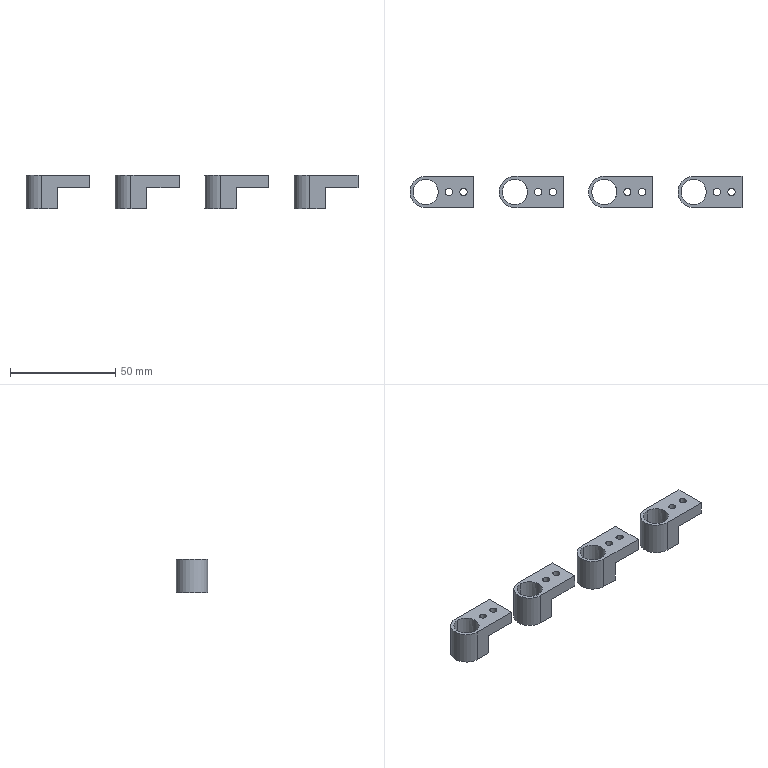NC program | NX | posted with a generic post | part box 158 x 15 x 16 mm
Lines 1 to 59 of 6389:
N10 G17 G21 G94 G90
(FLOOR_WALL , TOOL : D63)
N12 T03 M6
N14 G54
N16 G17 G0 G90 X-116.5 Y0. S6500 M3
N18 G43 Z30. H3
N20 Z3.
N22 G94 G1 Z0. F1500.
N24 X-113.5
N26 X113.5
N28 X116.5
N30 Z3.
N32 G0 Z30.
N34 M5
(DRILLING , TOOL : D6A45)
N36 T01 M6
N38 G54
N40 G17 G0 G90 X-71.5 Y0. S5000 M3
N42 G43 Z30. H1
N44 G94 G81 G98 Z-1. F250. R3.
N46 X-60.5
N48 X-53.5
N50 X-29.
N52 X-18.
N54 X-11.
N56 X13.5
N58 X24.5
N60 X31.5
N62 X56.
N64 X67.
N66 X74.
N68 G80
N70 G0 X74. Y0. Z30.
N72 M5
(DRILLING_COPY , TOOL : 3.4ZT)
N74 T13 M6
N76 G54
N78 G17 G0 G90 X-71.5 Y0. S2000 M3
N80 G43 Z30. H13
N82 G94 G83 G98 Z-18.521 F150. Q2. R3.
N84 X-60.5 Z-8.521
N86 X-53.5
N88 X-29. Z-18.521
N90 X-18. Z-8.521
N92 X-11.
N94 X13.5 Z-18.521
N96 X24.5 Z-8.521
N98 X31.5
N100 G80
N102 G0 X31.5 Y0. Z30.
N104 M5